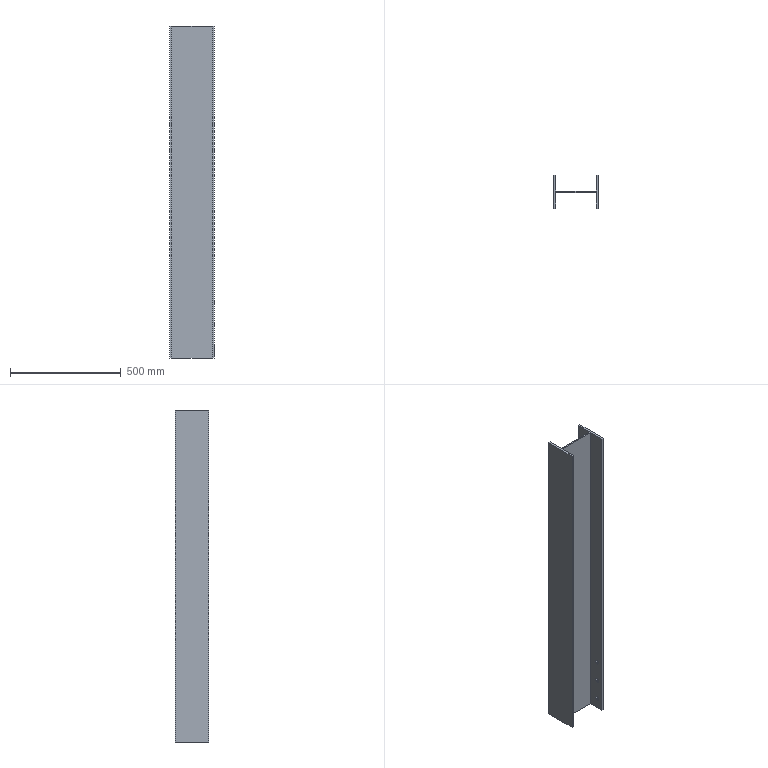Part | SolidWorks | features Extrusion 1, ICE 1 | 1 solid | 26 faces | box 200 x 150 x 1500 mm | volume 5674259 mm3 | plane 14 | cylinder 12 | commonest cylinder face diameters 18 x12
STEP:
#1=CARTESIAN_POINT('',(100.,-45.,241.));
#2=VERTEX_POINT('',#1);
#3=CARTESIAN_POINT('',(100.,-45.,259.));
#4=VERTEX_POINT('',#3);
#5=CARTESIAN_POINT('',(100.,-45.,250.));
#6=DIRECTION('',(-1.,0.,0.));
#7=DIRECTION('',(0.,-1.,0.));
#8=AXIS2_PLACEMENT_3D('',#5,#6,#7);
#9=CIRCLE('',#8,9.);
#10=EDGE_CURVE('',#2,#4,#9,.T.);
#11=ORIENTED_EDGE('',*,*,#10,.F.);
#12=CARTESIAN_POINT('',(91.,-45.,241.));
#13=VERTEX_POINT('',#12);
#14=CARTESIAN_POINT('',(1591.,-45.,241.));
#15=DIRECTION('',(-1.,0.,0.));
#16=VECTOR('',#15,1000.);
#17=LINE('',#14,#16);
#18=EDGE_CURVE('',#2,#13,#17,.T.);
#19=ORIENTED_EDGE('',*,*,#18,.T.);
#20=CARTESIAN_POINT('',(91.,-45.,259.));
#21=VERTEX_POINT('',#20);
#22=CARTESIAN_POINT('',(91.,-45.,250.));
#23=DIRECTION('',(-1.,0.,0.));
#24=DIRECTION('',(0.,0.,1.));
#25=AXIS2_PLACEMENT_3D('',#22,#23,#24);
#26=CIRCLE('',#25,9.);
#27=EDGE_CURVE('',#13,#21,#26,.T.);
#28=ORIENTED_EDGE('',*,*,#27,.T.);
#29=CARTESIAN_POINT('',(1591.,-45.,259.));
#30=DIRECTION('',(-1.,0.,0.));
#31=VECTOR('',#30,1000.);
#32=LINE('',#29,#31);
#33=EDGE_CURVE('',#4,#21,#32,.T.);
#34=ORIENTED_EDGE('',*,*,#33,.F.);
#35=EDGE_LOOP('',(#11,#19,#28,#34));
#36=FACE_OUTER_BOUND('',#35,.T.);
#37=CARTESIAN_POINT('',(1591.,-45.,250.));
#38=DIRECTION('',(-1.,0.,0.));
#39=DIRECTION('',(0.,0.,1.));
#40=AXIS2_PLACEMENT_3D('',#37,#38,#39);
#41=CYLINDRICAL_SURFACE('',#40,9.);
#42=ADVANCED_FACE('',(#36),#41,.F.);
#43=CARTESIAN_POINT('',(100.,-45.,141.));
#44=VERTEX_POINT('',#43);
#45=CARTESIAN_POINT('',(100.,-45.,159.));
#46=VERTEX_POINT('',#45);
#47=CARTESIAN_POINT('',(100.,-45.,150.));
#48=DIRECTION('',(-1.,0.,0.));
#49=DIRECTION('',(0.,-1.,0.));
#50=AXIS2_PLACEMENT_3D('',#47,#48,#49);
#51=CIRCLE('',#50,9.);
#52=EDGE_CURVE('',#44,#46,#51,.T.);
#53=ORIENTED_EDGE('',*,*,#52,.F.);
#54=CARTESIAN_POINT('',(91.,-45.,141.));
#55=VERTEX_POINT('',#54);
#56=CARTESIAN_POINT('',(1591.,-45.,141.));
#57=DIRECTION('',(-1.,0.,0.));
#58=VECTOR('',#57,1000.);
#59=LINE('',#56,#58);
#60=EDGE_CURVE('',#44,#55,#59,.T.);
#61=ORIENTED_EDGE('',*,*,#60,.T.);
#62=CARTESIAN_POINT('',(91.,-45.,159.));
#63=VERTEX_POINT('',#62);
#64=CARTESIAN_POINT('',(91.,-45.,150.));
#65=DIRECTION('',(-1.,0.,0.));
#66=DIRECTION('',(0.,0.,1.));
#67=AXIS2_PLACEMENT_3D('',#64,#65,#66);
#68=CIRCLE('',#67,9.);
#69=EDGE_CURVE('',#55,#63,#68,.T.);
#70=ORIENTED_EDGE('',*,*,#69,.T.);
#71=CARTESIAN_POINT('',(1591.,-45.,159.));
#72=DIRECTION('',(-1.,0.,0.));
#73=VECTOR('',#72,1000.);
#74=LINE('',#71,#73);
#75=EDGE_CURVE('',#46,#63,#74,.T.);
#76=ORIENTED_EDGE('',*,*,#75,.F.);
#77=EDGE_LOOP('',(#53,#61,#70,#76));
#78=FACE_OUTER_BOUND('',#77,.T.);
#79=CARTESIAN_POINT('',(1591.,-45.,150.));
#80=DIRECTION('',(-1.,0.,0.));
#81=DIRECTION('',(0.,0.,1.));
#82=AXIS2_PLACEMENT_3D('',#79,#80,#81);
#83=CYLINDRICAL_SURFACE('',#82,9.);
#84=ADVANCED_FACE('',(#78),#83,.F.);
#85=CARTESIAN_POINT('',(100.,-45.,41.));
#86=VERTEX_POINT('',#85);
#87=CARTESIAN_POINT('',(100.,-45.,59.));
#88=VERTEX_POINT('',#87);
#89=CARTESIAN_POINT('',(100.,-45.,50.));
#90=DIRECTION('',(-1.,0.,0.));
#91=DIRECTION('',(0.,-1.,0.));
#92=AXIS2_PLACEMENT_3D('',#89,#90,#91);
#93=CIRCLE('',#92,9.);
#94=EDGE_CURVE('',#86,#88,#93,.T.);
#95=ORIENTED_EDGE('',*,*,#94,.F.);
#96=CARTESIAN_POINT('',(91.,-45.,41.));
#97=VERTEX_POINT('',#96);
#98=CARTESIAN_POINT('',(1591.,-45.,41.));
#99=DIRECTION('',(-1.,0.,0.));
#100=VECTOR('',#99,1000.);
#101=LINE('',#98,#100);
#102=EDGE_CURVE('',#86,#97,#101,.T.);
#103=ORIENTED_EDGE('',*,*,#102,.T.);
#104=CARTESIAN_POINT('',(91.,-45.,59.));
#105=VERTEX_POINT('',#104);
#106=CARTESIAN_POINT('',(91.,-45.,50.));
#107=DIRECTION('',(-1.,0.,0.));
#108=DIRECTION('',(0.,0.,1.));
#109=AXIS2_PLACEMENT_3D('',#106,#107,#108);
#110=CIRCLE('',#109,9.);
#111=EDGE_CURVE('',#97,#105,#110,.T.);
#112=ORIENTED_EDGE('',*,*,#111,.T.);
#113=CARTESIAN_POINT('',(1591.,-45.,59.));
#114=DIRECTION('',(-1.,0.,0.));
#115=VECTOR('',#114,1000.);
#116=LINE('',#113,#115);
#117=EDGE_CURVE('',#88,#105,#116,.T.);
#118=ORIENTED_EDGE('',*,*,#117,.F.);
#119=EDGE_LOOP('',(#95,#103,#112,#118));
#120=FACE_OUTER_BOUND('',#119,.T.);
#121=CARTESIAN_POINT('',(1591.,-45.,50.));
#122=DIRECTION('',(-1.,0.,0.));
#123=DIRECTION('',(0.,0.,1.));
#124=AXIS2_PLACEMENT_3D('',#121,#122,#123);
#125=CYLINDRICAL_SURFACE('',#124,9.);
#126=ADVANCED_FACE('',(#120),#125,.F.);
#127=CARTESIAN_POINT('',(100.,45.,41.));
#128=VERTEX_POINT('',#127);
#129=CARTESIAN_POINT('',(100.,45.,59.));
#130=VERTEX_POINT('',#129);
#131=CARTESIAN_POINT('',(100.,45.,50.));
#132=DIRECTION('',(-1.,0.,0.));
#133=DIRECTION('',(0.,-1.,0.));
#134=AXIS2_PLACEMENT_3D('',#131,#132,#133);
#135=CIRCLE('',#134,9.);
#136=EDGE_CURVE('',#128,#130,#135,.T.);
#137=ORIENTED_EDGE('',*,*,#136,.F.);
#138=CARTESIAN_POINT('',(91.,45.,41.));
#139=VERTEX_POINT('',#138);
#140=CARTESIAN_POINT('',(1591.,45.,41.));
#141=DIRECTION('',(-1.,0.,0.));
#142=VECTOR('',#141,1000.);
#143=LINE('',#140,#142);
#144=EDGE_CURVE('',#128,#139,#143,.T.);
#145=ORIENTED_EDGE('',*,*,#144,.T.);
#146=CARTESIAN_POINT('',(91.,45.,59.));
#147=VERTEX_POINT('',#146);
#148=CARTESIAN_POINT('',(91.,45.,50.));
#149=DIRECTION('',(-1.,0.,0.));
#150=DIRECTION('',(0.,0.,-1.));
#151=AXIS2_PLACEMENT_3D('',#148,#149,#150);
#152=CIRCLE('',#151,9.);
#153=EDGE_CURVE('',#139,#147,#152,.T.);
#154=ORIENTED_EDGE('',*,*,#153,.T.);
#155=CARTESIAN_POINT('',(1591.,45.,59.));
#156=DIRECTION('',(-1.,0.,0.));
#157=VECTOR('',#156,1000.);
#158=LINE('',#155,#157);
#159=EDGE_CURVE('',#130,#147,#158,.T.);
#160=ORIENTED_EDGE('',*,*,#159,.F.);
#161=EDGE_LOOP('',(#137,#145,#154,#160));
#162=FACE_OUTER_BOUND('',#161,.T.);
#163=CARTESIAN_POINT('',(1591.,45.,50.));
#164=DIRECTION('',(-1.,0.,0.));
#165=DIRECTION('',(0.,0.,1.));
#166=AXIS2_PLACEMENT_3D('',#163,#164,#165);
#167=CYLINDRICAL_SURFACE('',#166,9.);
#168=ADVANCED_FACE('',(#162),#167,.F.);
#169=CARTESIAN_POINT('',(100.,45.,141.));
#170=VERTEX_POINT('',#169);
#171=CARTESIAN_POINT('',(100.,45.,159.));
#172=VERTEX_POINT('',#171);
#173=CARTESIAN_POINT('',(100.,45.,150.));
#174=DIRECTION('',(-1.,0.,0.));
#175=DIRECTION('',(0.,-1.,0.));
#176=AXIS2_PLACEMENT_3D('',#173,#174,#175);
#177=CIRCLE('',#176,9.);
#178=EDGE_CURVE('',#170,#172,#177,.T.);
#179=ORIENTED_EDGE('',*,*,#178,.F.);
#180=CARTESIAN_POINT('',(91.,45.,141.));
#181=VERTEX_POINT('',#180);
#182=CARTESIAN_POINT('',(1591.,45.,141.));
#183=DIRECTION('',(-1.,0.,0.));
#184=VECTOR('',#183,1000.);
#185=LINE('',#182,#184);
#186=EDGE_CURVE('',#170,#181,#185,.T.);
#187=ORIENTED_EDGE('',*,*,#186,.T.);
#188=CARTESIAN_POINT('',(91.,45.,159.));
#189=VERTEX_POINT('',#188);
#190=CARTESIAN_POINT('',(91.,45.,150.));
#191=DIRECTION('',(-1.,0.,0.));
#192=DIRECTION('',(0.,0.,-1.));
#193=AXIS2_PLACEMENT_3D('',#190,#191,#192);
#194=CIRCLE('',#193,9.);
#195=EDGE_CURVE('',#181,#189,#194,.T.);
#196=ORIENTED_EDGE('',*,*,#195,.T.);
#197=CARTESIAN_POINT('',(1591.,45.,159.));
#198=DIRECTION('',(-1.,0.,0.));
#199=VECTOR('',#198,1000.);
#200=LINE('',#197,#199);
#201=EDGE_CURVE('',#172,#189,#200,.T.);
#202=ORIENTED_EDGE('',*,*,#201,.F.);
#203=EDGE_LOOP('',(#179,#187,#196,#202));
#204=FACE_OUTER_BOUND('',#203,.T.);
#205=CARTESIAN_POINT('',(1591.,45.,150.));
#206=DIRECTION('',(-1.,0.,0.));
#207=DIRECTION('',(0.,0.,1.));
#208=AXIS2_PLACEMENT_3D('',#205,#206,#207);
#209=CYLINDRICAL_SURFACE('',#208,9.);
#210=ADVANCED_FACE('',(#204),#209,.F.);
#211=CARTESIAN_POINT('',(100.,45.,241.));
#212=VERTEX_POINT('',#211);
#213=CARTESIAN_POINT('',(100.,45.,259.));
#214=VERTEX_POINT('',#213);
#215=CARTESIAN_POINT('',(100.,45.,250.));
#216=DIRECTION('',(-1.,0.,0.));
#217=DIRECTION('',(0.,-1.,0.));
#218=AXIS2_PLACEMENT_3D('',#215,#216,#217);
#219=CIRCLE('',#218,9.);
#220=EDGE_CURVE('',#212,#214,#219,.T.);
#221=ORIENTED_EDGE('',*,*,#220,.F.);
#222=CARTESIAN_POINT('',(91.,45.,241.));
#223=VERTEX_POINT('',#222);
#224=CARTESIAN_POINT('',(1591.,45.,241.));
#225=DIRECTION('',(-1.,0.,0.));
#226=VECTOR('',#225,1000.);
#227=LINE('',#224,#226);
#228=EDGE_CURVE('',#212,#223,#227,.T.);
#229=ORIENTED_EDGE('',*,*,#228,.T.);
#230=CARTESIAN_POINT('',(91.,45.,259.));
#231=VERTEX_POINT('',#230);
#232=CARTESIAN_POINT('',(91.,45.,250.));
#233=DIRECTION('',(-1.,0.,0.));
#234=DIRECTION('',(0.,0.,-1.));
#235=AXIS2_PLACEMENT_3D('',#232,#233,#234);
#236=CIRCLE('',#235,9.);
#237=EDGE_CURVE('',#223,#231,#236,.T.);
#238=ORIENTED_EDGE('',*,*,#237,.T.);
#239=CARTESIAN_POINT('',(1591.,45.,259.));
#240=DIRECTION('',(-1.,0.,0.));
#241=VECTOR('',#240,1000.);
#242=LINE('',#239,#241);
#243=EDGE_CURVE('',#214,#231,#242,.T.);
#244=ORIENTED_EDGE('',*,*,#243,.F.);
#245=EDGE_LOOP('',(#221,#229,#238,#244));
#246=FACE_OUTER_BOUND('',#245,.T.);
#247=CARTESIAN_POINT('',(1591.,45.,250.));
#248=DIRECTION('',(-1.,0.,0.));
#249=DIRECTION('',(0.,0.,1.));
#250=AXIS2_PLACEMENT_3D('',#247,#248,#249);
#251=CYLINDRICAL_SURFACE('',#250,9.);
#252=ADVANCED_FACE('',(#246),#251,.F.);
#253=CARTESIAN_POINT('',(-100.,75.,0.));
#254=VERTEX_POINT('',#253);
#255=CARTESIAN_POINT('',(-100.,-75.,0.));
#256=VERTEX_POINT('',#255);
#257=CARTESIAN_POINT('',(-100.,-75.,0.));
#258=DIRECTION('',(0.,-1.,0.));
#259=VECTOR('',#258,1000.);
#260=LINE('',#257,#259);
#261=EDGE_CURVE('',#254,#256,#260,.T.);
#262=ORIENTED_EDGE('',*,*,#261,.T.);
#263=CARTESIAN_POINT('',(-100.,-75.,1500.));
#264=VERTEX_POINT('',#263);
#265=CARTESIAN_POINT('',(-100.,-75.,1500.));
#266=DIRECTION('',(0.,0.,-1.));
#267=VECTOR('',#266,1000.);
#268=LINE('',#265,#267);
#269=EDGE_CURVE('',#264,#256,#268,.T.);
#270=ORIENTED_EDGE('',*,*,#269,.F.);
#271=CARTESIAN_POINT('',(-100.,75.,1500.));
#272=VERTEX_POINT('',#271);
#273=CARTESIAN_POINT('',(-100.,-75.,1500.));
#274=DIRECTION('',(0.,-1.,0.));
#275=VECTOR('',#274,1000.);
#276=LINE('',#273,#275);
#277=EDGE_CURVE('',#272,#264,#276,.T.);
#278=ORIENTED_EDGE('',*,*,#277,.F.);
#279=CARTESIAN_POINT('',(-100.,75.,1500.));
#280=DIRECTION('',(0.,0.,-1.));
#281=VECTOR('',#280,1000.);
#282=LINE('',#279,#281);
#283=EDGE_CURVE('',#272,#254,#282,.T.);
#284=ORIENTED_EDGE('',*,*,#283,.T.);
#285=EDGE_LOOP('',(#262,#270,#278,#284));
#286=FACE_OUTER_BOUND('',#285,.T.);
#287=CARTESIAN_POINT('',(-100.,-75.,1500.));
#288=DIRECTION('',(1.,0.,0.));
#289=DIRECTION('',(0.,1.,0.));
#290=AXIS2_PLACEMENT_3D('',#287,#288,#289);
#291=PLANE('',#290);
#292=ADVANCED_FACE('',(#286),#291,.F.);
#293=CARTESIAN_POINT('',(-91.,-75.,0.));
#294=VERTEX_POINT('',#293);
#295=CARTESIAN_POINT('',(-91.,-75.,0.));
#296=DIRECTION('',(1.,0.,0.));
#297=VECTOR('',#296,1000.);
#298=LINE('',#295,#297);
#299=EDGE_CURVE('',#256,#294,#298,.T.);
#300=ORIENTED_EDGE('',*,*,#299,.T.);
#301=CARTESIAN_POINT('',(-91.,-75.,1500.));
#302=VERTEX_POINT('',#301);
#303=CARTESIAN_POINT('',(-91.,-75.,1500.));
#304=DIRECTION('',(0.,0.,-1.));
#305=VECTOR('',#304,1000.);
#306=LINE('',#303,#305);
#307=EDGE_CURVE('',#302,#294,#306,.T.);
#308=ORIENTED_EDGE('',*,*,#307,.F.);
#309=CARTESIAN_POINT('',(-91.,-75.,1500.));
#310=DIRECTION('',(1.,0.,0.));
#311=VECTOR('',#310,1000.);
#312=LINE('',#309,#311);
#313=EDGE_CURVE('',#264,#302,#312,.T.);
#314=ORIENTED_EDGE('',*,*,#313,.F.);
#315=ORIENTED_EDGE('',*,*,#269,.T.);
#316=EDGE_LOOP('',(#300,#308,#314,#315));
#317=FACE_OUTER_BOUND('',#316,.T.);
#318=CARTESIAN_POINT('',(-91.,-75.,1500.));
#319=DIRECTION('',(0.,1.,0.));
#320=DIRECTION('',(0.,0.,1.));
#321=AXIS2_PLACEMENT_3D('',#318,#319,#320);
#322=PLANE('',#321);
#323=ADVANCED_FACE('',(#317),#322,.F.);
#324=CARTESIAN_POINT('',(-91.,-3.,0.));
#325=VERTEX_POINT('',#324);
#326=CARTESIAN_POINT('',(-91.,-75.,0.));
#327=DIRECTION('',(0.,1.,0.));
#328=VECTOR('',#327,1000.);
#329=LINE('',#326,#328);
#330=EDGE_CURVE('',#294,#325,#329,.T.);
#331=ORIENTED_EDGE('',*,*,#330,.T.);
#332=CARTESIAN_POINT('',(-91.,-3.,1500.));
#333=VERTEX_POINT('',#332);
#334=CARTESIAN_POINT('',(-91.,-3.,1500.));
#335=DIRECTION('',(0.,0.,-1.));
#336=VECTOR('',#335,1000.);
#337=LINE('',#334,#336);
#338=EDGE_CURVE('',#333,#325,#337,.T.);
#339=ORIENTED_EDGE('',*,*,#338,.F.);
#340=CARTESIAN_POINT('',(-91.,-75.,1500.));
#341=DIRECTION('',(0.,1.,0.));
#342=VECTOR('',#341,1000.);
#343=LINE('',#340,#342);
#344=EDGE_CURVE('',#302,#333,#343,.T.);
#345=ORIENTED_EDGE('',*,*,#344,.F.);
#346=ORIENTED_EDGE('',*,*,#307,.T.);
#347=EDGE_LOOP('',(#331,#339,#345,#346));
#348=FACE_OUTER_BOUND('',#347,.T.);
#349=CARTESIAN_POINT('',(-91.,-75.,1500.));
#350=DIRECTION('',(-1.,0.,0.));
#351=DIRECTION('',(0.,0.,1.));
#352=AXIS2_PLACEMENT_3D('',#349,#350,#351);
#353=PLANE('',#352);
#354=ADVANCED_FACE('',(#348),#353,.F.);
#355=CARTESIAN_POINT('',(91.,-3.,0.));
#356=VERTEX_POINT('',#355);
#357=CARTESIAN_POINT('',(91.,-3.,0.));
#358=DIRECTION('',(1.,0.,0.));
#359=VECTOR('',#358,1000.);
#360=LINE('',#357,#359);
#361=EDGE_CURVE('',#325,#356,#360,.T.);
#362=ORIENTED_EDGE('',*,*,#361,.T.);
#363=CARTESIAN_POINT('',(91.,-3.,1500.));
#364=VERTEX_POINT('',#363);
#365=CARTESIAN_POINT('',(91.,-3.,1500.));
#366=DIRECTION('',(0.,0.,-1.));
#367=VECTOR('',#366,1000.);
#368=LINE('',#365,#367);
#369=EDGE_CURVE('',#364,#356,#368,.T.);
#370=ORIENTED_EDGE('',*,*,#369,.F.);
#371=CARTESIAN_POINT('',(91.,-3.,1500.));
#372=DIRECTION('',(1.,0.,0.));
#373=VECTOR('',#372,1000.);
#374=LINE('',#371,#373);
#375=EDGE_CURVE('',#333,#364,#374,.T.);
#376=ORIENTED_EDGE('',*,*,#375,.F.);
#377=ORIENTED_EDGE('',*,*,#338,.T.);
#378=EDGE_LOOP('',(#362,#370,#376,#377));
#379=FACE_OUTER_BOUND('',#378,.T.);
#380=CARTESIAN_POINT('',(91.,-3.,1500.));
#381=DIRECTION('',(0.,1.,0.));
#382=DIRECTION('',(-1.,0.,0.));
#383=AXIS2_PLACEMENT_3D('',#380,#381,#382);
#384=PLANE('',#383);
#385=ADVANCED_FACE('',(#379),#384,.F.);
#386=CARTESIAN_POINT('',(91.,-45.,250.));
#387=DIRECTION('',(-1.,0.,0.));
#388=DIRECTION('',(0.,0.,1.));
#389=AXIS2_PLACEMENT_3D('',#386,#387,#388);
#390=CIRCLE('',#389,9.);
#391=EDGE_CURVE('',#21,#13,#390,.T.);
#392=ORIENTED_EDGE('',*,*,#391,.F.);
#393=ORIENTED_EDGE('',*,*,#27,.F.);
#394=EDGE_LOOP('',(#392,#393));
#395=FACE_BOUND('',#394,.T.);
#396=CARTESIAN_POINT('',(91.,-45.,150.));
#397=DIRECTION('',(-1.,0.,0.));
#398=DIRECTION('',(0.,0.,1.));
#399=AXIS2_PLACEMENT_3D('',#396,#397,#398);
#400=CIRCLE('',#399,9.);
#401=EDGE_CURVE('',#63,#55,#400,.T.);
#402=ORIENTED_EDGE('',*,*,#401,.F.);
#403=ORIENTED_EDGE('',*,*,#69,.F.);
#404=EDGE_LOOP('',(#402,#403));
#405=FACE_BOUND('',#404,.T.);
#406=CARTESIAN_POINT('',(91.,-45.,50.));
#407=DIRECTION('',(-1.,0.,0.));
#408=DIRECTION('',(0.,0.,1.));
#409=AXIS2_PLACEMENT_3D('',#406,#407,#408);
#410=CIRCLE('',#409,9.);
#411=EDGE_CURVE('',#105,#97,#410,.T.);
#412=ORIENTED_EDGE('',*,*,#411,.F.);
#413=ORIENTED_EDGE('',*,*,#111,.F.);
#414=EDGE_LOOP('',(#412,#413));
#415=FACE_BOUND('',#414,.T.);
#416=CARTESIAN_POINT('',(91.,-75.,0.));
#417=VERTEX_POINT('',#416);
#418=CARTESIAN_POINT('',(91.,-75.,0.));
#419=DIRECTION('',(0.,-1.,0.));
#420=VECTOR('',#419,1000.);
#421=LINE('',#418,#420);
#422=EDGE_CURVE('',#356,#417,#421,.T.);
#423=ORIENTED_EDGE('',*,*,#422,.T.);
#424=CARTESIAN_POINT('',(91.,-75.,1500.));
#425=VERTEX_POINT('',#424);
#426=CARTESIAN_POINT('',(91.,-75.,1500.));
#427=DIRECTION('',(0.,0.,-1.));
#428=VECTOR('',#427,1000.);
#429=LINE('',#426,#428);
#430=EDGE_CURVE('',#425,#417,#429,.T.);
#431=ORIENTED_EDGE('',*,*,#430,.F.);
#432=CARTESIAN_POINT('',(91.,-75.,1500.));
#433=DIRECTION('',(0.,-1.,0.));
#434=VECTOR('',#433,1000.);
#435=LINE('',#432,#434);
#436=EDGE_CURVE('',#364,#425,#435,.T.);
#437=ORIENTED_EDGE('',*,*,#436,.F.);
#438=ORIENTED_EDGE('',*,*,#369,.T.);
#439=EDGE_LOOP('',(#423,#431,#437,#438));
#440=FACE_OUTER_BOUND('',#439,.T.);
#441=CARTESIAN_POINT('',(91.,-75.,1500.));
#442=DIRECTION('',(1.,0.,0.));
#443=DIRECTION('',(0.,0.,-1.));
#444=AXIS2_PLACEMENT_3D('',#441,#442,#443);
#445=PLANE('',#444);
#446=ADVANCED_FACE('',(#395,#405,#415,#440),#445,.F.);
#447=CARTESIAN_POINT('',(100.,-75.,0.));
#448=VERTEX_POINT('',#447);
#449=CARTESIAN_POINT('',(91.,-75.,0.));
#450=DIRECTION('',(1.,0.,0.));
#451=VECTOR('',#450,1000.);
#452=LINE('',#449,#451);
#453=EDGE_CURVE('',#417,#448,#452,.T.);
#454=ORIENTED_EDGE('',*,*,#453,.T.);
#455=CARTESIAN_POINT('',(100.,-75.,1500.));
#456=VERTEX_POINT('',#455);
#457=CARTESIAN_POINT('',(100.,-75.,1500.));
#458=DIRECTION('',(0.,0.,-1.));
#459=VECTOR('',#458,1000.);
#460=LINE('',#457,#459);
#461=EDGE_CURVE('',#456,#448,#460,.T.);
#462=ORIENTED_EDGE('',*,*,#461,.F.);
#463=CARTESIAN_POINT('',(91.,-75.,1500.));
#464=DIRECTION('',(1.,0.,0.));
#465=VECTOR('',#464,1000.);
#466=LINE('',#463,#465);
#467=EDGE_CURVE('',#425,#456,#466,.T.);
#468=ORIENTED_EDGE('',*,*,#467,.F.);
#469=ORIENTED_EDGE('',*,*,#430,.T.);
#470=EDGE_LOOP('',(#454,#462,#468,#469));
#471=FACE_OUTER_BOUND('',#470,.T.);
#472=CARTESIAN_POINT('',(91.,-75.,1500.));
#473=DIRECTION('',(0.,1.,0.));
#474=DIRECTION('',(0.,0.,1.));
#475=AXIS2_PLACEMENT_3D('',#472,#473,#474);
#476=PLANE('',#475);
#477=ADVANCED_FACE('',(#471),#476,.F.);
#478=CARTESIAN_POINT('',(100.,45.,50.));
#479=DIRECTION('',(-1.,0.,0.));
#480=DIRECTION('',(0.,-1.,0.));
#481=AXIS2_PLACEMENT_3D('',#478,#479,#480);
#482=CIRCLE('',#481,9.);
#483=EDGE_CURVE('',#130,#128,#482,.T.);
#484=ORIENTED_EDGE('',*,*,#483,.T.);
#485=ORIENTED_EDGE('',*,*,#136,.T.);
#486=EDGE_LOOP('',(#484,#485));
#487=FACE_BOUND('',#486,.T.);
#488=CARTESIAN_POINT('',(100.,45.,150.));
#489=DIRECTION('',(-1.,0.,0.));
#490=DIRECTION('',(0.,-1.,0.));
#491=AXIS2_PLACEMENT_3D('',#488,#489,#490);
#492=CIRCLE('',#491,9.);
#493=EDGE_CURVE('',#172,#170,#492,.T.);
#494=ORIENTED_EDGE('',*,*,#493,.T.);
#495=ORIENTED_EDGE('',*,*,#178,.T.);
#496=EDGE_LOOP('',(#494,#495));
#497=FACE_BOUND('',#496,.T.);
#498=CARTESIAN_POINT('',(100.,45.,250.));
#499=DIRECTION('',(-1.,0.,0.));
#500=DIRECTION('',(0.,-1.,0.));
#501=AXIS2_PLACEMENT_3D('',#498,#499,#500);
#502=CIRCLE('',#501,9.);
#503=EDGE_CURVE('',#214,#212,#502,.T.);
#504=ORIENTED_EDGE('',*,*,#503,.T.);
#505=ORIENTED_EDGE('',*,*,#220,.T.);
#506=EDGE_LOOP('',(#504,#505));
#507=FACE_BOUND('',#506,.T.);
#508=CARTESIAN_POINT('',(100.,-45.,250.));
#509=DIRECTION('',(-1.,0.,0.));
#510=DIRECTION('',(0.,-1.,0.));
#511=AXIS2_PLACEMENT_3D('',#508,#509,#510);
#512=CIRCLE('',#511,9.);
#513=EDGE_CURVE('',#4,#2,#512,.T.);
#514=ORIENTED_EDGE('',*,*,#513,.T.);
#515=ORIENTED_EDGE('',*,*,#10,.T.);
#516=EDGE_LOOP('',(#514,#515));
#517=FACE_BOUND('',#516,.T.);
#518=CARTESIAN_POINT('',(100.,-45.,150.));
#519=DIRECTION('',(-1.,0.,0.));
#520=DIRECTION('',(0.,-1.,0.));
#521=AXIS2_PLACEMENT_3D('',#518,#519,#520);
#522=CIRCLE('',#521,9.);
#523=EDGE_CURVE('',#46,#44,#522,.T.);
#524=ORIENTED_EDGE('',*,*,#523,.T.);
#525=ORIENTED_EDGE('',*,*,#52,.T.);
#526=EDGE_LOOP('',(#524,#525));
#527=FACE_BOUND('',#526,.T.);
#528=CARTESIAN_POINT('',(100.,-45.,50.));
#529=DIRECTION('',(-1.,0.,0.));
#530=DIRECTION('',(0.,-1.,0.));
#531=AXIS2_PLACEMENT_3D('',#528,#529,#530);
#532=CIRCLE('',#531,9.);
#533=EDGE_CURVE('',#88,#86,#532,.T.);
#534=ORIENTED_EDGE('',*,*,#533,.T.);
#535=ORIENTED_EDGE('',*,*,#94,.T.);
#536=EDGE_LOOP('',(#534,#535));
#537=FACE_BOUND('',#536,.T.);
#538=CARTESIAN_POINT('',(100.,75.,0.));
#539=VERTEX_POINT('',#538);
#540=CARTESIAN_POINT('',(100.,-75.,0.));
#541=DIRECTION('',(0.,1.,0.));
#542=VECTOR('',#541,1000.);
#543=LINE('',#540,#542);
#544=EDGE_CURVE('',#448,#539,#543,.T.);
#545=ORIENTED_EDGE('',*,*,#544,.T.);
#546=CARTESIAN_POINT('',(100.,75.,1500.));
#547=VERTEX_POINT('',#546);
#548=CARTESIAN_POINT('',(100.,75.,1500.));
#549=DIRECTION('',(0.,0.,-1.));
#550=VECTOR('',#549,1000.);
#551=LINE('',#548,#550);
#552=EDGE_CURVE('',#547,#539,#551,.T.);
#553=ORIENTED_EDGE('',*,*,#552,.F.);
#554=CARTESIAN_POINT('',(100.,-75.,1500.));
#555=DIRECTION('',(0.,1.,0.));
#556=VECTOR('',#555,1000.);
#557=LINE('',#554,#556);
#558=EDGE_CURVE('',#456,#547,#557,.T.);
#559=ORIENTED_EDGE('',*,*,#558,.F.);
#560=ORIENTED_EDGE('',*,*,#461,.T.);
#561=EDGE_LOOP('',(#545,#553,#559,#560));
#562=FACE_OUTER_BOUND('',#561,.T.);
#563=CARTESIAN_POINT('',(100.,-75.,1500.));
#564=DIRECTION('',(-1.,0.,0.));
#565=DIRECTION('',(0.,-1.,0.));
#566=AXIS2_PLACEMENT_3D('',#563,#564,#565);
#567=PLANE('',#566);
#568=ADVANCED_FACE('',(#487,#497,#507,#517,#527,#537,#562),#567,.F.);
#569=CARTESIAN_POINT('',(91.,75.,0.));
#570=VERTEX_POINT('',#569);
#571=CARTESIAN_POINT('',(91.,75.,0.));
#572=DIRECTION('',(-1.,0.,0.));
#573=VECTOR('',#572,1000.);
#574=LINE('',#571,#573);
#575=EDGE_CURVE('',#539,#570,#574,.T.);
#576=ORIENTED_EDGE('',*,*,#575,.T.);
#577=CARTESIAN_POINT('',(91.,75.,1500.));
#578=VERTEX_POINT('',#577);
#579=CARTESIAN_POINT('',(91.,75.,1500.));
#580=DIRECTION('',(0.,0.,-1.));
#581=VECTOR('',#580,1000.);
#582=LINE('',#579,#581);
#583=EDGE_CURVE('',#578,#570,#582,.T.);
#584=ORIENTED_EDGE('',*,*,#583,.F.);
#585=CARTESIAN_POINT('',(91.,75.,1500.));
#586=DIRECTION('',(-1.,0.,0.));
#587=VECTOR('',#586,1000.);
#588=LINE('',#585,#587);
#589=EDGE_CURVE('',#547,#578,#588,.T.);
#590=ORIENTED_EDGE('',*,*,#589,.F.);
#591=ORIENTED_EDGE('',*,*,#552,.T.);
#592=EDGE_LOOP('',(#576,#584,#590,#591));
#593=FACE_OUTER_BOUND('',#592,.T.);
#594=CARTESIAN_POINT('',(91.,75.,1500.));
#595=DIRECTION('',(0.,-1.,0.));
#596=DIRECTION('',(0.,0.,-1.));
#597=AXIS2_PLACEMENT_3D('',#594,#595,#596);
#598=PLANE('',#597);
#599=ADVANCED_FACE('',(#593),#598,.F.);
#600=CARTESIAN_POINT('',(91.,45.,50.));
#601=DIRECTION('',(-1.,0.,0.));
#602=DIRECTION('',(0.,0.,-1.));
#603=AXIS2_PLACEMENT_3D('',#600,#601,#602);
#604=CIRCLE('',#603,9.);
#605=EDGE_CURVE('',#147,#139,#604,.T.);
#606=ORIENTED_EDGE('',*,*,#605,.F.);
#607=ORIENTED_EDGE('',*,*,#153,.F.);
#608=EDGE_LOOP('',(#606,#607));
#609=FACE_BOUND('',#608,.T.);
#610=CARTESIAN_POINT('',(91.,45.,150.));
#611=DIRECTION('',(-1.,0.,0.));
#612=DIRECTION('',(0.,0.,-1.));
#613=AXIS2_PLACEMENT_3D('',#610,#611,#612);
#614=CIRCLE('',#613,9.);
#615=EDGE_CURVE('',#189,#181,#614,.T.);
#616=ORIENTED_EDGE('',*,*,#615,.F.);
#617=ORIENTED_EDGE('',*,*,#195,.F.);
#618=EDGE_LOOP('',(#616,#617));
#619=FACE_BOUND('',#618,.T.);
#620=CARTESIAN_POINT('',(91.,45.,250.));
#621=DIRECTION('',(-1.,0.,0.));
#622=DIRECTION('',(0.,0.,-1.));
#623=AXIS2_PLACEMENT_3D('',#620,#621,#622);
#624=CIRCLE('',#623,9.);
#625=EDGE_CURVE('',#231,#223,#624,.T.);
#626=ORIENTED_EDGE('',*,*,#625,.F.);
#627=ORIENTED_EDGE('',*,*,#237,.F.);
#628=EDGE_LOOP('',(#626,#627));
#629=FACE_BOUND('',#628,.T.);
#630=CARTESIAN_POINT('',(91.,3.,0.));
#631=VERTEX_POINT('',#630);
#632=CARTESIAN_POINT('',(91.,3.,0.));
#633=DIRECTION('',(0.,-1.,0.));
#634=VECTOR('',#633,1000.);
#635=LINE('',#632,#634);
#636=EDGE_CURVE('',#570,#631,#635,.T.);
#637=ORIENTED_EDGE('',*,*,#636,.T.);
#638=CARTESIAN_POINT('',(91.,3.,1500.));
#639=VERTEX_POINT('',#638);
#640=CARTESIAN_POINT('',(91.,3.,1500.));
#641=DIRECTION('',(0.,0.,-1.));
#642=VECTOR('',#641,1000.);
#643=LINE('',#640,#642);
#644=EDGE_CURVE('',#639,#631,#643,.T.);
#645=ORIENTED_EDGE('',*,*,#644,.F.);
#646=CARTESIAN_POINT('',(91.,3.,1500.));
#647=DIRECTION('',(0.,-1.,0.));
#648=VECTOR('',#647,1000.);
#649=LINE('',#646,#648);
#650=EDGE_CURVE('',#578,#639,#649,.T.);
#651=ORIENTED_EDGE('',*,*,#650,.F.);
#652=ORIENTED_EDGE('',*,*,#583,.T.);
#653=EDGE_LOOP('',(#637,#645,#651,#652));
#654=FACE_OUTER_BOUND('',#653,.T.);
#655=CARTESIAN_POINT('',(91.,3.,1500.));
#656=DIRECTION('',(1.,0.,0.));
#657=DIRECTION('',(0.,0.,-1.));
#658=AXIS2_PLACEMENT_3D('',#655,#656,#657);
#659=PLANE('',#658);
#660=ADVANCED_FACE('',(#609,#619,#629,#654),#659,.F.);
#661=CARTESIAN_POINT('',(-91.,3.,0.));
#662=VERTEX_POINT('',#661);
#663=CARTESIAN_POINT('',(91.,3.,0.));
#664=DIRECTION('',(-1.,0.,0.));
#665=VECTOR('',#664,1000.);
#666=LINE('',#663,#665);
#667=EDGE_CURVE('',#631,#662,#666,.T.);
#668=ORIENTED_EDGE('',*,*,#667,.T.);
#669=CARTESIAN_POINT('',(-91.,3.,1500.));
#670=VERTEX_POINT('',#669);
#671=CARTESIAN_POINT('',(-91.,3.,1500.));
#672=DIRECTION('',(0.,0.,-1.));
#673=VECTOR('',#672,1000.);
#674=LINE('',#671,#673);
#675=EDGE_CURVE('',#670,#662,#674,.T.);
#676=ORIENTED_EDGE('',*,*,#675,.F.);
#677=CARTESIAN_POINT('',(91.,3.,1500.));
#678=DIRECTION('',(-1.,0.,0.));
#679=VECTOR('',#678,1000.);
#680=LINE('',#677,#679);
#681=EDGE_CURVE('',#639,#670,#680,.T.);
#682=ORIENTED_EDGE('',*,*,#681,.F.);
#683=ORIENTED_EDGE('',*,*,#644,.T.);
#684=EDGE_LOOP('',(#668,#676,#682,#683));
#685=FACE_OUTER_BOUND('',#684,.T.);
#686=CARTESIAN_POINT('',(91.,3.,1500.));
#687=DIRECTION('',(0.,-1.,0.));
#688=DIRECTION('',(0.,0.,-1.));
#689=AXIS2_PLACEMENT_3D('',#686,#687,#688);
#690=PLANE('',#689);
#691=ADVANCED_FACE('',(#685),#690,.F.);
#692=CARTESIAN_POINT('',(-91.,75.,0.));
#693=VERTEX_POINT('',#692);
#694=CARTESIAN_POINT('',(-91.,3.,0.));
#695=DIRECTION('',(0.,1.,0.));
#696=VECTOR('',#695,1000.);
#697=LINE('',#694,#696);
#698=EDGE_CURVE('',#662,#693,#697,.T.);
#699=ORIENTED_EDGE('',*,*,#698,.T.);
#700=CARTESIAN_POINT('',(-91.,75.,1500.));
#701=VERTEX_POINT('',#700);
#702=CARTESIAN_POINT('',(-91.,75.,1500.));
#703=DIRECTION('',(0.,0.,-1.));
#704=VECTOR('',#703,1000.);
#705=LINE('',#702,#704);
#706=EDGE_CURVE('',#701,#693,#705,.T.);
#707=ORIENTED_EDGE('',*,*,#706,.F.);
#708=CARTESIAN_POINT('',(-91.,3.,1500.));
#709=DIRECTION('',(0.,1.,0.));
#710=VECTOR('',#709,1000.);
#711=LINE('',#708,#710);
#712=EDGE_CURVE('',#670,#701,#711,.T.);
#713=ORIENTED_EDGE('',*,*,#712,.F.);
#714=ORIENTED_EDGE('',*,*,#675,.T.);
#715=EDGE_LOOP('',(#699,#707,#713,#714));
#716=FACE_OUTER_BOUND('',#715,.T.);
#717=CARTESIAN_POINT('',(-91.,3.,1500.));
#718=DIRECTION('',(-1.,0.,0.));
#719=DIRECTION('',(0.,0.,1.));
#720=AXIS2_PLACEMENT_3D('',#717,#718,#719);
#721=PLANE('',#720);
#722=ADVANCED_FACE('',(#716),#721,.F.);
#723=CARTESIAN_POINT('',(-91.,75.,0.));
#724=DIRECTION('',(-1.,0.,0.));
#725=VECTOR('',#724,1000.);
#726=LINE('',#723,#725);
#727=EDGE_CURVE('',#693,#254,#726,.T.);
#728=ORIENTED_EDGE('',*,*,#727,.T.);
#729=ORIENTED_EDGE('',*,*,#283,.F.);
#730=CARTESIAN_POINT('',(-91.,75.,1500.));
#731=DIRECTION('',(-1.,0.,0.));
#732=VECTOR('',#731,1000.);
#733=LINE('',#730,#732);
#734=EDGE_CURVE('',#701,#272,#733,.T.);
#735=ORIENTED_EDGE('',*,*,#734,.F.);
#736=ORIENTED_EDGE('',*,*,#706,.T.);
#737=EDGE_LOOP('',(#728,#729,#735,#736));
#738=FACE_OUTER_BOUND('',#737,.T.);
#739=CARTESIAN_POINT('',(-91.,75.,1500.));
#740=DIRECTION('',(0.,-1.,0.));
#741=DIRECTION('',(0.,0.,-1.));
#742=AXIS2_PLACEMENT_3D('',#739,#740,#741);
#743=PLANE('',#742);
#744=ADVANCED_FACE('',(#738),#743,.F.);
#745=ORIENTED_EDGE('',*,*,#277,.T.);
#746=ORIENTED_EDGE('',*,*,#313,.T.);
#747=ORIENTED_EDGE('',*,*,#344,.T.);
#748=ORIENTED_EDGE('',*,*,#375,.T.);
#749=ORIENTED_EDGE('',*,*,#436,.T.);
#750=ORIENTED_EDGE('',*,*,#467,.T.);
#751=ORIENTED_EDGE('',*,*,#558,.T.);
#752=ORIENTED_EDGE('',*,*,#589,.T.);
#753=ORIENTED_EDGE('',*,*,#650,.T.);
#754=ORIENTED_EDGE('',*,*,#681,.T.);
#755=ORIENTED_EDGE('',*,*,#712,.T.);
#756=ORIENTED_EDGE('',*,*,#734,.T.);
#757=EDGE_LOOP('',(#745,#746,#747,#748,#749,#750,#751,#752,#753,#754,#755,#756));
#758=FACE_OUTER_BOUND('',#757,.T.);
#759=CARTESIAN_POINT('',(0.,0.,1500.));
#760=DIRECTION('',(0.,0.,1.));
#761=DIRECTION('',(1.,0.,0.));
#762=AXIS2_PLACEMENT_3D('',#759,#760,#761);
#763=PLANE('',#762);
#764=ADVANCED_FACE('',(#758),#763,.T.);
#765=ORIENTED_EDGE('',*,*,#261,.F.);
#766=ORIENTED_EDGE('',*,*,#727,.F.);
#767=ORIENTED_EDGE('',*,*,#698,.F.);
#768=ORIENTED_EDGE('',*,*,#667,.F.);
#769=ORIENTED_EDGE('',*,*,#636,.F.);
#770=ORIENTED_EDGE('',*,*,#575,.F.);
#771=ORIENTED_EDGE('',*,*,#544,.F.);
#772=ORIENTED_EDGE('',*,*,#453,.F.);
#773=ORIENTED_EDGE('',*,*,#422,.F.);
#774=ORIENTED_EDGE('',*,*,#361,.F.);
#775=ORIENTED_EDGE('',*,*,#330,.F.);
#776=ORIENTED_EDGE('',*,*,#299,.F.);
#777=EDGE_LOOP('',(#765,#766,#767,#768,#769,#770,#771,#772,#773,#774,#775,#776));
#778=FACE_OUTER_BOUND('',#777,.T.);
#779=CARTESIAN_POINT('',(0.,0.,0.));
#780=DIRECTION('',(0.,0.,1.));
#781=DIRECTION('',(1.,0.,0.));
#782=AXIS2_PLACEMENT_3D('',#779,#780,#781);
#783=PLANE('',#782);
#784=ADVANCED_FACE('',(#778),#783,.F.);
#785=ORIENTED_EDGE('',*,*,#228,.F.);
#786=ORIENTED_EDGE('',*,*,#503,.F.);
#787=ORIENTED_EDGE('',*,*,#243,.T.);
#788=ORIENTED_EDGE('',*,*,#625,.T.);
#789=EDGE_LOOP('',(#785,#786,#787,#788));
#790=FACE_OUTER_BOUND('',#789,.T.);
#791=CARTESIAN_POINT('',(1591.,45.,250.));
#792=DIRECTION('',(-1.,0.,0.));
#793=DIRECTION('',(0.,0.,1.));
#794=AXIS2_PLACEMENT_3D('',#791,#792,#793);
#795=CYLINDRICAL_SURFACE('',#794,9.);
#796=ADVANCED_FACE('',(#790),#795,.F.);
#797=ORIENTED_EDGE('',*,*,#186,.F.);
#798=ORIENTED_EDGE('',*,*,#493,.F.);
#799=ORIENTED_EDGE('',*,*,#201,.T.);
#800=ORIENTED_EDGE('',*,*,#615,.T.);
#801=EDGE_LOOP('',(#797,#798,#799,#800));
#802=FACE_OUTER_BOUND('',#801,.T.);
#803=CARTESIAN_POINT('',(1591.,45.,150.));
#804=DIRECTION('',(-1.,0.,0.));
#805=DIRECTION('',(0.,0.,1.));
#806=AXIS2_PLACEMENT_3D('',#803,#804,#805);
#807=CYLINDRICAL_SURFACE('',#806,9.);
#808=ADVANCED_FACE('',(#802),#807,.F.);
#809=ORIENTED_EDGE('',*,*,#144,.F.);
#810=ORIENTED_EDGE('',*,*,#483,.F.);
#811=ORIENTED_EDGE('',*,*,#159,.T.);
#812=ORIENTED_EDGE('',*,*,#605,.T.);
#813=EDGE_LOOP('',(#809,#810,#811,#812));
#814=FACE_OUTER_BOUND('',#813,.T.);
#815=CARTESIAN_POINT('',(1591.,45.,50.));
#816=DIRECTION('',(-1.,0.,0.));
#817=DIRECTION('',(0.,0.,1.));
#818=AXIS2_PLACEMENT_3D('',#815,#816,#817);
#819=CYLINDRICAL_SURFACE('',#818,9.);
#820=ADVANCED_FACE('',(#814),#819,.F.);
#821=ORIENTED_EDGE('',*,*,#102,.F.);
#822=ORIENTED_EDGE('',*,*,#533,.F.);
#823=ORIENTED_EDGE('',*,*,#117,.T.);
#824=ORIENTED_EDGE('',*,*,#411,.T.);
#825=EDGE_LOOP('',(#821,#822,#823,#824));
#826=FACE_OUTER_BOUND('',#825,.T.);
#827=CARTESIAN_POINT('',(1591.,-45.,50.));
#828=DIRECTION('',(-1.,0.,0.));
#829=DIRECTION('',(0.,0.,1.));
#830=AXIS2_PLACEMENT_3D('',#827,#828,#829);
#831=CYLINDRICAL_SURFACE('',#830,9.);
#832=ADVANCED_FACE('',(#826),#831,.F.);
#833=ORIENTED_EDGE('',*,*,#60,.F.);
#834=ORIENTED_EDGE('',*,*,#523,.F.);
#835=ORIENTED_EDGE('',*,*,#75,.T.);
#836=ORIENTED_EDGE('',*,*,#401,.T.);
#837=EDGE_LOOP('',(#833,#834,#835,#836));
#838=FACE_OUTER_BOUND('',#837,.T.);
#839=CARTESIAN_POINT('',(1591.,-45.,150.));
#840=DIRECTION('',(-1.,0.,0.));
#841=DIRECTION('',(0.,0.,1.));
#842=AXIS2_PLACEMENT_3D('',#839,#840,#841);
#843=CYLINDRICAL_SURFACE('',#842,9.);
#844=ADVANCED_FACE('',(#838),#843,.F.);
#845=ORIENTED_EDGE('',*,*,#18,.F.);
#846=ORIENTED_EDGE('',*,*,#513,.F.);
#847=ORIENTED_EDGE('',*,*,#33,.T.);
#848=ORIENTED_EDGE('',*,*,#391,.T.);
#849=EDGE_LOOP('',(#845,#846,#847,#848));
#850=FACE_OUTER_BOUND('',#849,.T.);
#851=CARTESIAN_POINT('',(1591.,-45.,250.));
#852=DIRECTION('',(-1.,0.,0.));
#853=DIRECTION('',(0.,0.,1.));
#854=AXIS2_PLACEMENT_3D('',#851,#852,#853);
#855=CYLINDRICAL_SURFACE('',#854,9.);
#856=ADVANCED_FACE('',(#850),#855,.F.);
#857=CLOSED_SHELL('',(#42,#84,#126,#168,#210,#252,#292,#323,#354,#385,#446,#477,#568,#599,#660,#691,#722,#744,#764,#784,#796,#808,#820,#832,#844,#856));
#858=MANIFOLD_SOLID_BREP('',#857);
#859=CARTESIAN_POINT('',(0.,0.,0.));
#860=DIRECTION('',(0.,0.,1.));
#861=DIRECTION('',(1.,0.,0.));
#862=AXIS2_PLACEMENT_3D('',#859,#860,#861);
#863=(LENGTH_UNIT()NAMED_UNIT(*)SI_UNIT(.MILLI.,.METRE.));
#864=UNCERTAINTY_MEASURE_WITH_UNIT(LENGTH_MEASURE(0.00001),#863,'','');
#865=(NAMED_UNIT(*)PLANE_ANGLE_UNIT()SI_UNIT($,.RADIAN.));
#866=(NAMED_UNIT(*)SI_UNIT($,.STERADIAN.)SOLID_ANGLE_UNIT());
#867=(GEOMETRIC_REPRESENTATION_CONTEXT(3)GLOBAL_UNCERTAINTY_ASSIGNED_CONTEXT((#864))GLOBAL_UNIT_ASSIGNED_CONTEXT((#863,#865,#866))REPRESENTATION_CONTEXT('',''));
#868=ADVANCED_BREP_SHAPE_REPRESENTATION('',(#858,#862),#867);